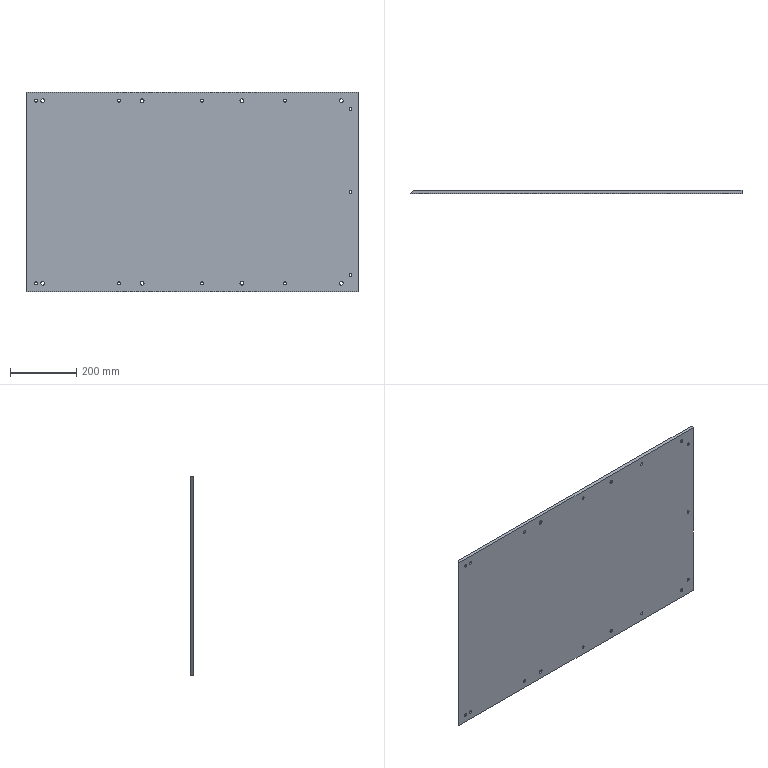Part | STEP file | PN_0039_cover plate_default_machined_ | 1 solid | 60 faces | box 1000 x 10 x 600 mm | volume 5952324 mm3 | cylinder 38 | cone 16 | plane 6 | commonest cylinder face diameters 8.5 x22 11 x16